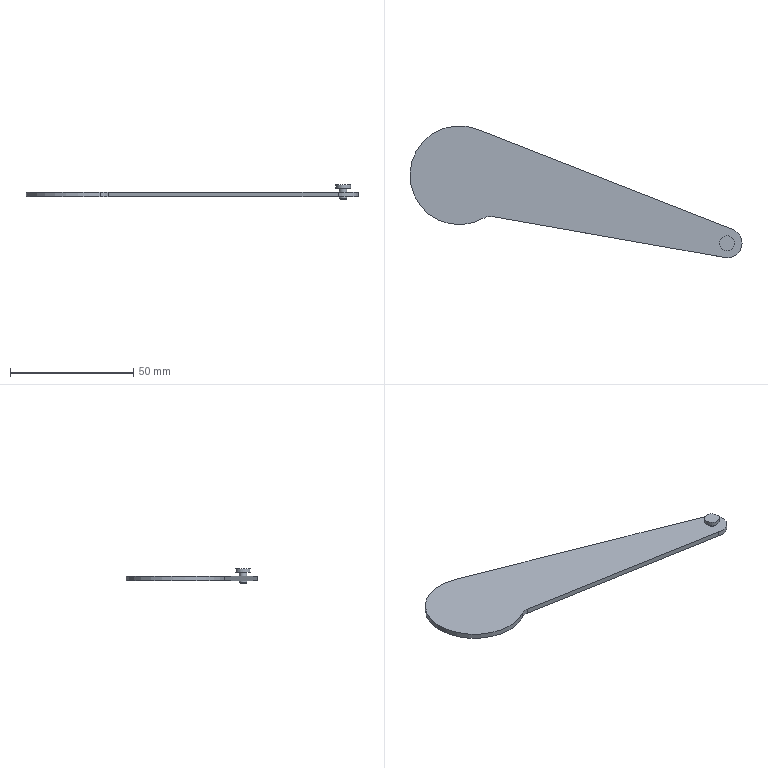Part | NX | 1 solid | 14 faces | box 134.5 x 53.5 x 6 mm | volume 6743 mm3 | plane 7 | cylinder 6 | cone 1 | commonest cylinder face diameters 3 x2 6 x1 10 x1 12 x1 40 x1
STEP:
#1=CARTESIAN_POINT('',(7.3,46.12,2.));
#2=VERTEX_POINT('',#1);
#3=CARTESIAN_POINT('',(10.001,10.18,2.));
#4=VERTEX_POINT('',#3);
#5=CARTESIAN_POINT('',(0.,27.5,2.));
#6=DIRECTION('',(0.,0.,1.));
#7=DIRECTION('',(1.,0.,0.));
#8=AXIS2_PLACEMENT_3D('',#5,#6,#7);
#9=CIRCLE('',#8,20.);
#10=EDGE_CURVE('',#2,#4,#9,.T.);
#11=ORIENTED_EDGE('',*,*,#10,.T.);
#12=CARTESIAN_POINT('',(13.369,10.774,2.));
#13=VERTEX_POINT('',#12);
#14=CARTESIAN_POINT('',(12.501,5.85,2.));
#15=DIRECTION('',(0.,0.,-1.));
#16=DIRECTION('',(-1.,0.,0.));
#17=AXIS2_PLACEMENT_3D('',#14,#15,#16);
#18=CIRCLE('',#17,5.);
#19=EDGE_CURVE('',#4,#13,#18,.T.);
#20=ORIENTED_EDGE('',*,*,#19,.T.);
#21=CARTESIAN_POINT('',(106.448,-5.638,2.));
#22=VERTEX_POINT('',#21);
#23=CARTESIAN_POINT('',(13.369,10.774,2.));
#24=DIRECTION('',(0.9848,-0.1736,0.));
#25=VECTOR('',#24,1000.);
#26=LINE('',#23,#25);
#27=EDGE_CURVE('',#13,#22,#26,.T.);
#28=ORIENTED_EDGE('',*,*,#27,.T.);
#29=CARTESIAN_POINT('',(110.69,5.586,2.));
#30=VERTEX_POINT('',#29);
#31=CARTESIAN_POINT('',(108.5,0.,2.));
#32=DIRECTION('',(0.,0.,1.));
#33=DIRECTION('',(1.,0.,0.));
#34=AXIS2_PLACEMENT_3D('',#31,#32,#33);
#35=CIRCLE('',#34,6.);
#36=EDGE_CURVE('',#22,#30,#35,.T.);
#37=ORIENTED_EDGE('',*,*,#36,.T.);
#38=CARTESIAN_POINT('',(110.69,5.586,2.));
#39=DIRECTION('',(-0.931,0.365,0.));
#40=VECTOR('',#39,1000.);
#41=LINE('',#38,#40);
#42=EDGE_CURVE('',#30,#2,#41,.T.);
#43=ORIENTED_EDGE('',*,*,#42,.T.);
#44=EDGE_LOOP('',(#11,#20,#28,#37,#43));
#45=FACE_BOUND('',#44,.T.);
#46=CARTESIAN_POINT('',(110.,0.,2.));
#47=VERTEX_POINT('',#46);
#48=CARTESIAN_POINT('',(108.5,0.,2.));
#49=DIRECTION('',(0.,0.,1.));
#50=DIRECTION('',(1.,0.,0.));
#51=AXIS2_PLACEMENT_3D('',#48,#49,#50);
#52=CIRCLE('',#51,1.5);
#53=EDGE_CURVE('',#47,#47,#52,.F.);
#54=ORIENTED_EDGE('',*,*,#53,.T.);
#55=EDGE_LOOP('',(#54));
#56=FACE_BOUND('',#55,.T.);
#57=CARTESIAN_POINT('',(0.,27.5,2.));
#58=DIRECTION('',(0.,0.,1.));
#59=DIRECTION('',(1.,0.,0.));
#60=AXIS2_PLACEMENT_3D('',#57,#58,#59);
#61=PLANE('',#60);
#62=ADVANCED_FACE('',(#45,#56),#61,.T.);
#63=CARTESIAN_POINT('',(7.3,46.12,0.));
#64=VERTEX_POINT('',#63);
#65=CARTESIAN_POINT('',(10.001,10.18,0.));
#66=VERTEX_POINT('',#65);
#67=CARTESIAN_POINT('',(0.,27.5,0.));
#68=DIRECTION('',(0.,0.,1.));
#69=DIRECTION('',(1.,0.,0.));
#70=AXIS2_PLACEMENT_3D('',#67,#68,#69);
#71=CIRCLE('',#70,20.);
#72=EDGE_CURVE('',#64,#66,#71,.T.);
#73=ORIENTED_EDGE('',*,*,#72,.F.);
#74=CARTESIAN_POINT('',(110.69,5.586,0.));
#75=VERTEX_POINT('',#74);
#76=CARTESIAN_POINT('',(110.69,5.586,0.));
#77=DIRECTION('',(-0.931,0.365,0.));
#78=VECTOR('',#77,1000.);
#79=LINE('',#76,#78);
#80=EDGE_CURVE('',#75,#64,#79,.T.);
#81=ORIENTED_EDGE('',*,*,#80,.F.);
#82=CARTESIAN_POINT('',(106.448,-5.638,0.));
#83=VERTEX_POINT('',#82);
#84=CARTESIAN_POINT('',(108.5,0.,0.));
#85=DIRECTION('',(0.,0.,1.));
#86=DIRECTION('',(1.,0.,0.));
#87=AXIS2_PLACEMENT_3D('',#84,#85,#86);
#88=CIRCLE('',#87,6.);
#89=EDGE_CURVE('',#83,#75,#88,.T.);
#90=ORIENTED_EDGE('',*,*,#89,.F.);
#91=CARTESIAN_POINT('',(13.369,10.774,0.));
#92=VERTEX_POINT('',#91);
#93=CARTESIAN_POINT('',(13.369,10.774,0.));
#94=DIRECTION('',(0.9848,-0.1736,0.));
#95=VECTOR('',#94,1000.);
#96=LINE('',#93,#95);
#97=EDGE_CURVE('',#92,#83,#96,.T.);
#98=ORIENTED_EDGE('',*,*,#97,.F.);
#99=CARTESIAN_POINT('',(12.501,5.85,0.));
#100=DIRECTION('',(0.,0.,-1.));
#101=DIRECTION('',(-1.,0.,0.));
#102=AXIS2_PLACEMENT_3D('',#99,#100,#101);
#103=CIRCLE('',#102,5.);
#104=EDGE_CURVE('',#66,#92,#103,.T.);
#105=ORIENTED_EDGE('',*,*,#104,.F.);
#106=EDGE_LOOP('',(#73,#81,#90,#98,#105));
#107=FACE_BOUND('',#106,.T.);
#108=CARTESIAN_POINT('',(110.,0.,0.));
#109=VERTEX_POINT('',#108);
#110=CARTESIAN_POINT('',(108.5,0.,0.));
#111=DIRECTION('',(0.,0.,1.));
#112=DIRECTION('',(1.,0.,0.));
#113=AXIS2_PLACEMENT_3D('',#110,#111,#112);
#114=CIRCLE('',#113,1.5);
#115=EDGE_CURVE('',#109,#109,#114,.F.);
#116=ORIENTED_EDGE('',*,*,#115,.F.);
#117=EDGE_LOOP('',(#116));
#118=FACE_BOUND('',#117,.T.);
#119=CARTESIAN_POINT('',(0.,27.5,0.));
#120=DIRECTION('',(0.,0.,1.));
#121=DIRECTION('',(1.,0.,0.));
#122=AXIS2_PLACEMENT_3D('',#119,#120,#121);
#123=PLANE('',#122);
#124=ADVANCED_FACE('',(#107,#118),#123,.F.);
#125=ORIENTED_EDGE('',*,*,#72,.T.);
#126=CARTESIAN_POINT('',(10.001,10.18,2.));
#127=DIRECTION('',(0.,0.,-1.));
#128=VECTOR('',#127,1000.);
#129=LINE('',#126,#128);
#130=EDGE_CURVE('',#4,#66,#129,.T.);
#131=ORIENTED_EDGE('',*,*,#130,.F.);
#132=ORIENTED_EDGE('',*,*,#10,.F.);
#133=CARTESIAN_POINT('',(7.3,46.12,2.));
#134=DIRECTION('',(0.,0.,-1.));
#135=VECTOR('',#134,1000.);
#136=LINE('',#133,#135);
#137=EDGE_CURVE('',#2,#64,#136,.T.);
#138=ORIENTED_EDGE('',*,*,#137,.T.);
#139=EDGE_LOOP('',(#125,#131,#132,#138));
#140=FACE_BOUND('',#139,.T.);
#141=CARTESIAN_POINT('',(0.,27.5,2.));
#142=DIRECTION('',(0.,0.,-1.));
#143=DIRECTION('',(-1.,0.,0.));
#144=AXIS2_PLACEMENT_3D('',#141,#142,#143);
#145=CYLINDRICAL_SURFACE('',#144,20.);
#146=ADVANCED_FACE('',(#140),#145,.T.);
#147=ORIENTED_EDGE('',*,*,#104,.T.);
#148=CARTESIAN_POINT('',(13.369,10.774,2.));
#149=DIRECTION('',(0.,0.,-1.));
#150=VECTOR('',#149,1000.);
#151=LINE('',#148,#150);
#152=EDGE_CURVE('',#13,#92,#151,.T.);
#153=ORIENTED_EDGE('',*,*,#152,.F.);
#154=ORIENTED_EDGE('',*,*,#19,.F.);
#155=ORIENTED_EDGE('',*,*,#130,.T.);
#156=EDGE_LOOP('',(#147,#153,#154,#155));
#157=FACE_BOUND('',#156,.T.);
#158=CARTESIAN_POINT('',(12.501,5.85,2.));
#159=DIRECTION('',(0.,0.,-1.));
#160=DIRECTION('',(-1.,0.,0.));
#161=AXIS2_PLACEMENT_3D('',#158,#159,#160);
#162=CYLINDRICAL_SURFACE('',#161,5.);
#163=ADVANCED_FACE('',(#157),#162,.F.);
#164=ORIENTED_EDGE('',*,*,#97,.T.);
#165=CARTESIAN_POINT('',(106.448,-5.638,2.));
#166=DIRECTION('',(0.,0.,-1.));
#167=VECTOR('',#166,1000.);
#168=LINE('',#165,#167);
#169=EDGE_CURVE('',#22,#83,#168,.T.);
#170=ORIENTED_EDGE('',*,*,#169,.F.);
#171=ORIENTED_EDGE('',*,*,#27,.F.);
#172=ORIENTED_EDGE('',*,*,#152,.T.);
#173=EDGE_LOOP('',(#164,#170,#171,#172));
#174=FACE_BOUND('',#173,.T.);
#175=CARTESIAN_POINT('',(13.369,10.774,2.));
#176=DIRECTION('',(0.1736,0.9848,0.));
#177=DIRECTION('',(-0.9848,0.1736,0.));
#178=AXIS2_PLACEMENT_3D('',#175,#176,#177);
#179=PLANE('',#178);
#180=ADVANCED_FACE('',(#174),#179,.F.);
#181=ORIENTED_EDGE('',*,*,#89,.T.);
#182=CARTESIAN_POINT('',(110.69,5.586,2.));
#183=DIRECTION('',(0.,0.,-1.));
#184=VECTOR('',#183,1000.);
#185=LINE('',#182,#184);
#186=EDGE_CURVE('',#30,#75,#185,.T.);
#187=ORIENTED_EDGE('',*,*,#186,.F.);
#188=ORIENTED_EDGE('',*,*,#36,.F.);
#189=ORIENTED_EDGE('',*,*,#169,.T.);
#190=EDGE_LOOP('',(#181,#187,#188,#189));
#191=FACE_BOUND('',#190,.T.);
#192=CARTESIAN_POINT('',(108.5,0.,2.));
#193=DIRECTION('',(0.,0.,-1.));
#194=DIRECTION('',(-1.,0.,0.));
#195=AXIS2_PLACEMENT_3D('',#192,#193,#194);
#196=CYLINDRICAL_SURFACE('',#195,6.);
#197=ADVANCED_FACE('',(#191),#196,.T.);
#198=ORIENTED_EDGE('',*,*,#80,.T.);
#199=ORIENTED_EDGE('',*,*,#137,.F.);
#200=ORIENTED_EDGE('',*,*,#42,.F.);
#201=ORIENTED_EDGE('',*,*,#186,.T.);
#202=EDGE_LOOP('',(#198,#199,#200,#201));
#203=FACE_BOUND('',#202,.T.);
#204=CARTESIAN_POINT('',(110.69,5.586,2.));
#205=DIRECTION('',(-0.365,-0.931,0.));
#206=DIRECTION('',(0.931,-0.365,0.));
#207=AXIS2_PLACEMENT_3D('',#204,#205,#206);
#208=PLANE('',#207);
#209=ADVANCED_FACE('',(#203),#208,.F.);
#210=CARTESIAN_POINT('',(109.7,0.,-1.));
#211=VERTEX_POINT('',#210);
#212=CARTESIAN_POINT('',(108.5,0.,-1.));
#213=DIRECTION('',(0.,0.,1.));
#214=DIRECTION('',(1.,0.,0.));
#215=AXIS2_PLACEMENT_3D('',#212,#213,#214);
#216=CIRCLE('',#215,1.2);
#217=EDGE_CURVE('',#211,#211,#216,.T.);
#218=ORIENTED_EDGE('',*,*,#217,.F.);
#219=EDGE_LOOP('',(#218));
#220=FACE_BOUND('',#219,.T.);
#221=CARTESIAN_POINT('',(108.5,1.2,-1.));
#222=DIRECTION('',(0.,0.,1.));
#223=DIRECTION('',(1.,0.,0.));
#224=AXIS2_PLACEMENT_3D('',#221,#222,#223);
#225=PLANE('',#224);
#226=ADVANCED_FACE('',(#220),#225,.F.);
#227=CARTESIAN_POINT('',(110.,0.,-0.7));
#228=VERTEX_POINT('',#227);
#229=CARTESIAN_POINT('',(108.5,0.,-0.7));
#230=DIRECTION('',(0.,0.,1.));
#231=DIRECTION('',(1.,0.,0.));
#232=AXIS2_PLACEMENT_3D('',#229,#230,#231);
#233=CIRCLE('',#232,1.5);
#234=EDGE_CURVE('',#228,#228,#233,.T.);
#235=ORIENTED_EDGE('',*,*,#234,.F.);
#236=EDGE_LOOP('',(#235));
#237=FACE_BOUND('',#236,.T.);
#238=ORIENTED_EDGE('',*,*,#217,.T.);
#239=EDGE_LOOP('',(#238));
#240=FACE_BOUND('',#239,.T.);
#241=CARTESIAN_POINT('',(108.5,0.,-1.));
#242=DIRECTION('',(0.,0.,1.));
#243=DIRECTION('',(1.,0.,0.));
#244=AXIS2_PLACEMENT_3D('',#241,#242,#243);
#245=CONICAL_SURFACE('',#244,1.2,0.7854);
#246=ADVANCED_FACE('',(#237,#240),#245,.T.);
#247=ORIENTED_EDGE('',*,*,#234,.T.);
#248=EDGE_LOOP('',(#247));
#249=FACE_BOUND('',#248,.T.);
#250=ORIENTED_EDGE('',*,*,#115,.T.);
#251=EDGE_LOOP('',(#250));
#252=FACE_BOUND('',#251,.T.);
#253=CARTESIAN_POINT('',(108.5,0.,-1.));
#254=DIRECTION('',(0.,0.,1.));
#255=DIRECTION('',(1.,0.,0.));
#256=AXIS2_PLACEMENT_3D('',#253,#254,#255);
#257=CYLINDRICAL_SURFACE('',#256,1.5);
#258=ADVANCED_FACE('',(#249,#252),#257,.T.);
#259=CARTESIAN_POINT('',(111.5,0.,5.));
#260=VERTEX_POINT('',#259);
#261=CARTESIAN_POINT('',(108.5,0.,5.));
#262=DIRECTION('',(0.,0.,1.));
#263=DIRECTION('',(1.,0.,0.));
#264=AXIS2_PLACEMENT_3D('',#261,#262,#263);
#265=CIRCLE('',#264,3.);
#266=EDGE_CURVE('',#260,#260,#265,.T.);
#267=ORIENTED_EDGE('',*,*,#266,.T.);
#268=EDGE_LOOP('',(#267));
#269=FACE_BOUND('',#268,.T.);
#270=CARTESIAN_POINT('',(108.5,0.,5.));
#271=DIRECTION('',(0.,0.,-1.));
#272=DIRECTION('',(-1.,0.,0.));
#273=AXIS2_PLACEMENT_3D('',#270,#271,#272);
#274=PLANE('',#273);
#275=ADVANCED_FACE('',(#269),#274,.F.);
#276=ORIENTED_EDGE('',*,*,#266,.F.);
#277=EDGE_LOOP('',(#276));
#278=FACE_BOUND('',#277,.T.);
#279=CARTESIAN_POINT('',(111.5,0.,3.5));
#280=VERTEX_POINT('',#279);
#281=CARTESIAN_POINT('',(108.5,0.,3.5));
#282=DIRECTION('',(0.,0.,1.));
#283=DIRECTION('',(1.,0.,0.));
#284=AXIS2_PLACEMENT_3D('',#281,#282,#283);
#285=CIRCLE('',#284,3.);
#286=EDGE_CURVE('',#280,#280,#285,.T.);
#287=ORIENTED_EDGE('',*,*,#286,.T.);
#288=EDGE_LOOP('',(#287));
#289=FACE_BOUND('',#288,.T.);
#290=CARTESIAN_POINT('',(108.5,0.,-1.));
#291=DIRECTION('',(0.,0.,1.));
#292=DIRECTION('',(1.,0.,0.));
#293=AXIS2_PLACEMENT_3D('',#290,#291,#292);
#294=CYLINDRICAL_SURFACE('',#293,3.);
#295=ADVANCED_FACE('',(#278,#289),#294,.T.);
#296=ORIENTED_EDGE('',*,*,#286,.F.);
#297=EDGE_LOOP('',(#296));
#298=FACE_BOUND('',#297,.T.);
#299=CARTESIAN_POINT('',(110.,0.,3.5));
#300=VERTEX_POINT('',#299);
#301=CARTESIAN_POINT('',(108.5,0.,3.5));
#302=DIRECTION('',(0.,0.,1.));
#303=DIRECTION('',(1.,0.,0.));
#304=AXIS2_PLACEMENT_3D('',#301,#302,#303);
#305=CIRCLE('',#304,1.5);
#306=EDGE_CURVE('',#300,#300,#305,.T.);
#307=ORIENTED_EDGE('',*,*,#306,.T.);
#308=EDGE_LOOP('',(#307));
#309=FACE_BOUND('',#308,.T.);
#310=CARTESIAN_POINT('',(108.5,3.,3.5));
#311=DIRECTION('',(0.,0.,1.));
#312=DIRECTION('',(1.,0.,0.));
#313=AXIS2_PLACEMENT_3D('',#310,#311,#312);
#314=PLANE('',#313);
#315=ADVANCED_FACE('',(#298,#309),#314,.F.);
#316=ORIENTED_EDGE('',*,*,#53,.F.);
#317=EDGE_LOOP('',(#316));
#318=FACE_BOUND('',#317,.T.);
#319=ORIENTED_EDGE('',*,*,#306,.F.);
#320=EDGE_LOOP('',(#319));
#321=FACE_BOUND('',#320,.T.);
#322=CARTESIAN_POINT('',(108.5,0.,-1.));
#323=DIRECTION('',(0.,0.,1.));
#324=DIRECTION('',(1.,0.,0.));
#325=AXIS2_PLACEMENT_3D('',#322,#323,#324);
#326=CYLINDRICAL_SURFACE('',#325,1.5);
#327=ADVANCED_FACE('',(#318,#321),#326,.T.);
#328=CLOSED_SHELL('',(#62,#124,#146,#163,#180,#197,#209,#226,#246,#258,#275,#295,#315,#327));
#329=MANIFOLD_SOLID_BREP('',#328);
#330=(LENGTH_UNIT()NAMED_UNIT(*)SI_UNIT(.MILLI.,.METRE.));
#331=UNCERTAINTY_MEASURE_WITH_UNIT(LENGTH_MEASURE(0.00001),#330,'','');
#332=(NAMED_UNIT(*)PLANE_ANGLE_UNIT()SI_UNIT($,.RADIAN.));
#333=(NAMED_UNIT(*)SI_UNIT($,.STERADIAN.)SOLID_ANGLE_UNIT());
#334=(GEOMETRIC_REPRESENTATION_CONTEXT(3)GLOBAL_UNCERTAINTY_ASSIGNED_CONTEXT((#331))GLOBAL_UNIT_ASSIGNED_CONTEXT((#330,#332,#333))REPRESENTATION_CONTEXT('',''));
#335=ADVANCED_BREP_SHAPE_REPRESENTATION('',(#329),#334);